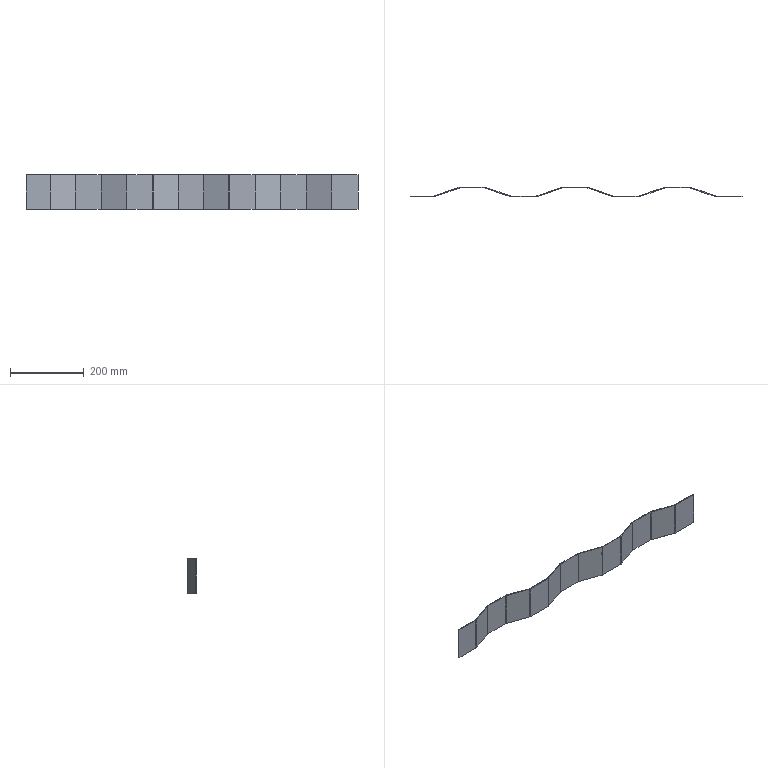Part | STEP file | 750038176 | 1 solid | 54 faces | box 900 x 26 x 92.5 mm | volume 171034 mm3 | plane 30 | cylinder 24 | commonest cylinder face diameters 6 x12 10 x12